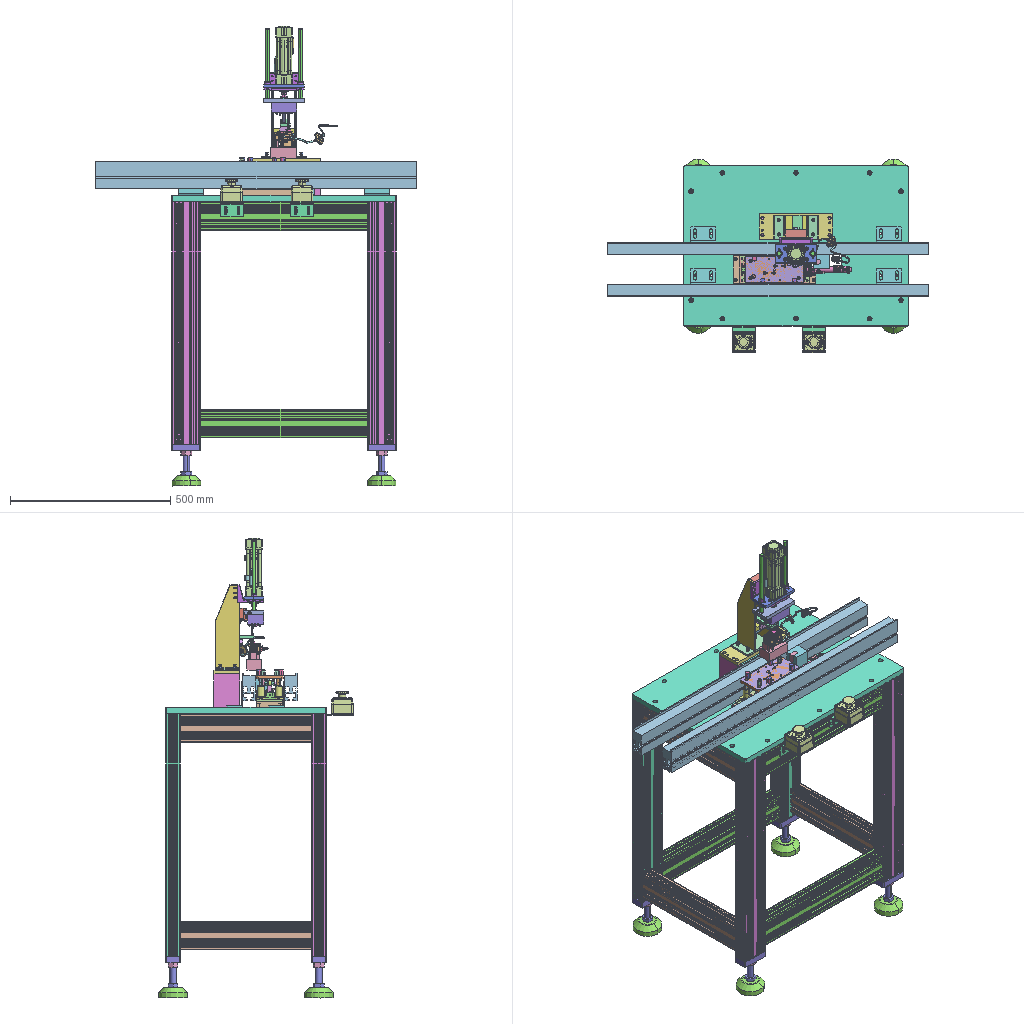Assembly | STEP file | 93 different items | 164 placed | box 1000 x 608 x 1437 mm
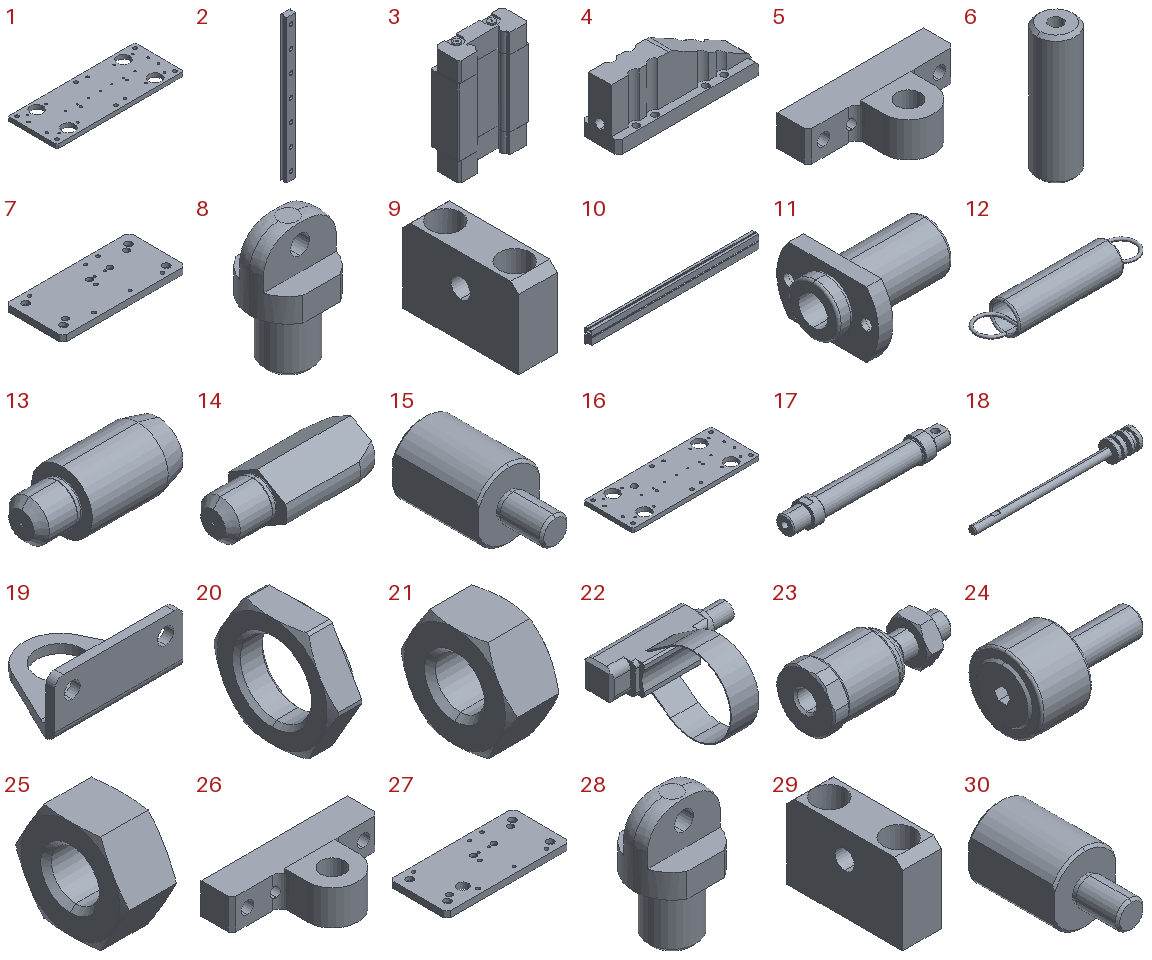Parts list (item | name | quantity | parent item | size | volume):
1 | PN_0007 | x1 | in lifting0012 | 220 x 85 x 7 mm | 118278 mm3
2 | STZL10_135 | x2 | in SE2BZ10_135_SE2BZ10-135 | 9 x 5.5 x 135 mm | 5384 mm3
3 | SEZB10 | x4 | in SE2BZ10_135_SE2BZ10-135 | 20 x 7.8 x 30 mm | 3504 mm3
4 | PN_0032 | x2 | in support001 | 75 x 20 x 31 mm | 24213 mm3
5 | PN_0022 | x1 | in lifting0012 | 38 x 21.5 x 9 mm | 3334 mm3
6 | PSFGT12-40-M5 | x4 | in lifting0012 | 12 x 12 x 40 mm | 4311 mm3
7 | PN_0010 | x1 | in lifting0012 | 180 x 84 x 9 mm | 130838 mm3
8 | PN_0039 | x2 | in lifting0012 | 8 x 7 x 13 mm | 305.811 mm3
9 | PN_0029 | x1 | in lifting0012 | 10 x 30 x 20 mm | 4165 mm3
10 | 8000-001 | x2 | in convvvvv | 1000 x 38.9 x 86 mm | 2174515 mm3
11 | LHICD12_LHICD12 | x8 | in lifting0012, PN_0033 | 47 x 42 x 27 mm | 14694 mm3
12 | AWA6_30_AWA6-30 | x3 | in lifting0012, PN_0033 | 31.1 x 6 x 6 mm | 196.407 mm3
13 | FPBA8_P12_L9_B15_FPBA8-P12-L8-B15 | x2 | in lifting0012, PN_0033 | 27 x 12 x 12 mm | 2448 mm3
14 | FPBD8_P12_L9_B15_FPBD8-P12-L9-B15 | x2 | in lifting0012, PN_0033 | 28 x 12 x 10.127 mm | 1917 mm3
15 | PN_0003 | x4 | in lifting0012 | 13 x 28.5 x 15 mm | 3349 mm3
16 | PN_0036 | x1 | in PN_0033 | 220 x 85 x 7 mm | 117728 mm3
17 | 16MALB50_Body | x1 | - | 142 x 21 x 21 mm | 18560 mm3
18 | 16LBMA50_Rod | x1 | - | 128 x 15.5 x 15.5 mm | 5968 mm3
19 | - | x1 | - | 44 x 32.5 x 19 mm | 4333 mm3
20 | 16_MA_Nut | x2 | - | 6 x 25 x 22 mm | 1467 mm3
21 | 16_MA_Nut1 | x1 | - | 5 x 11.547 x 10 mm | 331.027 mm3
22 | CS1_M_S16 | x2 | - | 30 x 26.6 x 17.8 mm | 1348 mm3
23 | F_M06100F_F-M06100F-P | x1 | in pull cylinder16 | 34.5 x 14.8 x 14 mm | 3405 mm3
24 | CFA6_16body | x1 | in CFA6_16_CFA6-16 | 28 x 16 x 16 mm | 2741 mm3
25 | nut_cua_6 | x1 | in CFA6_16_CFA6-16 | 5.2 x 11.547 x 10 mm | 345.699 mm3
26 | PN_0009 | x1 | in PN_0033 | 38 x 21.5 x 9 mm | 3334 mm3
27 | PN_0034 | x1 | in PN_0033 | 180 x 84 x 9 mm | 129247 mm3
28 | PN_0025 | x4 | in PN_0033 | 8 x 7 x 13 mm | 302.267 mm3
29 | PN_0030 | x1 | in PN_0033 | 10 x 30 x 20 mm | 4165 mm3
30 | PN_0015 | x4 | in PN_0033 | 13 x 28.5 x 15 mm | 3349 mm3
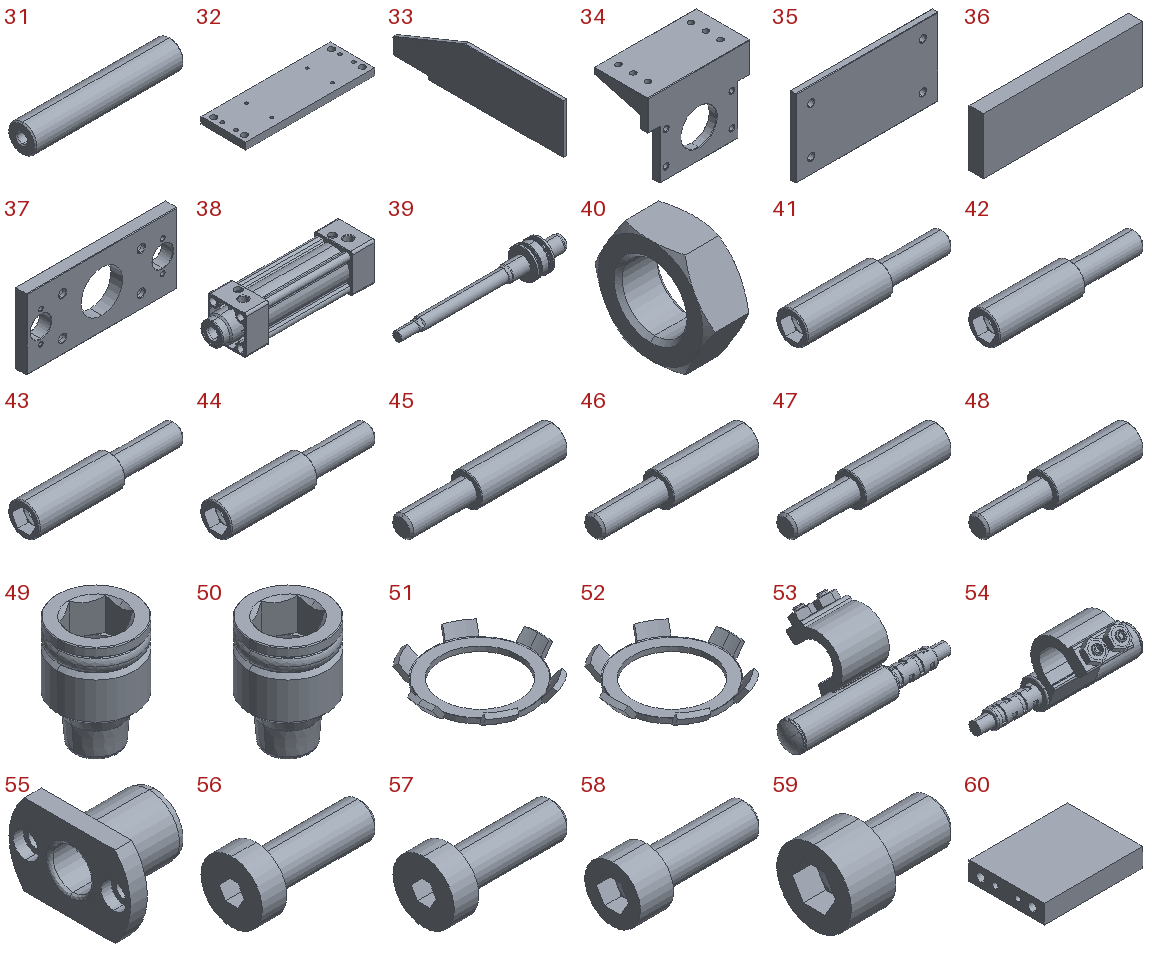31 | PSFGT12_64_M5_PSFGT12-64-M5 | x4 | in PN_0033 | 64 x 12 x 12 mm | 7075 mm3
32 | PN_0023 | x1 | in 10_ASM | 230 x 80 x 12 mm | 214344 mm3
33 | 1002 | x2 | in 10_ASM | - | -
34 | 1003 | x1 | in 10_ASM | 104 x 55 x 81 mm | 80858 mm3
35 | 10040 | x1 | in 10_ASM | 138 x 6 x 75 mm | 61187 mm3
36 | 1005 | x1 | in 10_ASM | 68 x 6 x 24 mm | 9792 mm3
37 | 1006 | x1 | in 10_ASM | 128 x 10 x 60 mm | 58293 mm3
38 | SI-40X75-S-B1N-2-1 | x1 | in SI-40X75-S-B1N-2_ASM | 204.5 x 53 x 53 mm | 210149 mm3
39 | SI-40X75-S-B1N-2-2 | x1 | in SI-40X75-S-B1N-2_ASM | 220.5 x 39.5 x 39.5 mm | 58608 mm3
40 | SI-40X75-S-B1N-2-3 | x1 | in SI-40X75-S-B1N-2_ASM | 7 x 19.63 x 17 mm | 1102 mm3
41 | SI-40X75-S-B1N-2-4 | x1 | in SI-40X75-S-B1N-2_ASM | 43 x 9 x 9 mm | 1649 mm3
42 | SI-40X75-S-B1N-2-5 | x1 | in SI-40X75-S-B1N-2_ASM | 43 x 9 x 9 mm | 1649 mm3
43 | SI-40X75-S-B1N-2-6 | x1 | in SI-40X75-S-B1N-2_ASM | 43 x 9 x 9 mm | 1649 mm3
44 | SI-40X75-S-B1N-2-7 | x1 | in SI-40X75-S-B1N-2_ASM | 43 x 9 x 9 mm | 1649 mm3
45 | SI-40X75-S-B1N-2-8 | x1 | in SI-40X75-S-B1N-2_ASM | 43 x 9 x 9 mm | 1649 mm3
46 | SI-40X75-S-B1N-2-9 | x1 | in SI-40X75-S-B1N-2_ASM | 43 x 9 x 9 mm | 1649 mm3
47 | SI-40X75-S-B1N-2-10 | x1 | in SI-40X75-S-B1N-2_ASM | 43 x 9 x 9 mm | 1649 mm3
48 | SI-40X75-S-B1N-2-11 | x1 | in SI-40X75-S-B1N-2_ASM | 43 x 9 x 9 mm | 1649 mm3
49 | SI-40X75-S-B1N-2-12 | x1 | in SI-40X75-S-B1N-2_ASM | 10 x 10 x 14.13 mm | 659.781 mm3
50 | SI-40X75-S-B1N-2-13 | x1 | in SI-40X75-S-B1N-2_ASM | 10 x 10 x 14.13 mm | 659.781 mm3
51 | SI-40X75-S-B1N-2-14 | x1 | in SI-40X75-S-B1N-2_ASM | 10 x 9.485 x 1.224 mm | 14.035 mm3
52 | SI-40X75-S-B1N-2-15 | x1 | in SI-40X75-S-B1N-2_ASM | 10 x 9.485 x 1.224 mm | 14.035 mm3
53 | SI-40X75-S-B1N-2-16 | x1 | in SI-40X75-S-B1N-2_ASM | 53.8 x 23.917 x 26.321 mm | 4702 mm3
54 | SI-40X75-S-B1N-2-17 | x1 | in SI-40X75-S-B1N-2_ASM | 53.8 x 23.917 x 26.321 mm | 4702 mm3
55 | SHTNZ12-25_1 | x2 | - | 25 x 36 x 24 mm | 5866 mm3
56 | SHTNZ12-25_2 | x2 | - | 14.8 x 7 x 7 mm | 244.398 mm3
57 | SHTNZ12-25_3 | x2 | - | 14.8 x 7 x 7 mm | 244.398 mm3
58 | CB6X1-L18-A10-E6-B5 | x6 | in 10_ASM, 20_ASM | 24 x 10 x 10 mm | 907.535 mm3
59 | CB6X1-10-A10-E6-B5 | x4 | in 10_ASM | 16 x 10 x 10 mm | 681.341 mm3
60 | PN_0028 | x2 | in 10_ASM | 105 x 80 x 20 mm | 160821 mm3
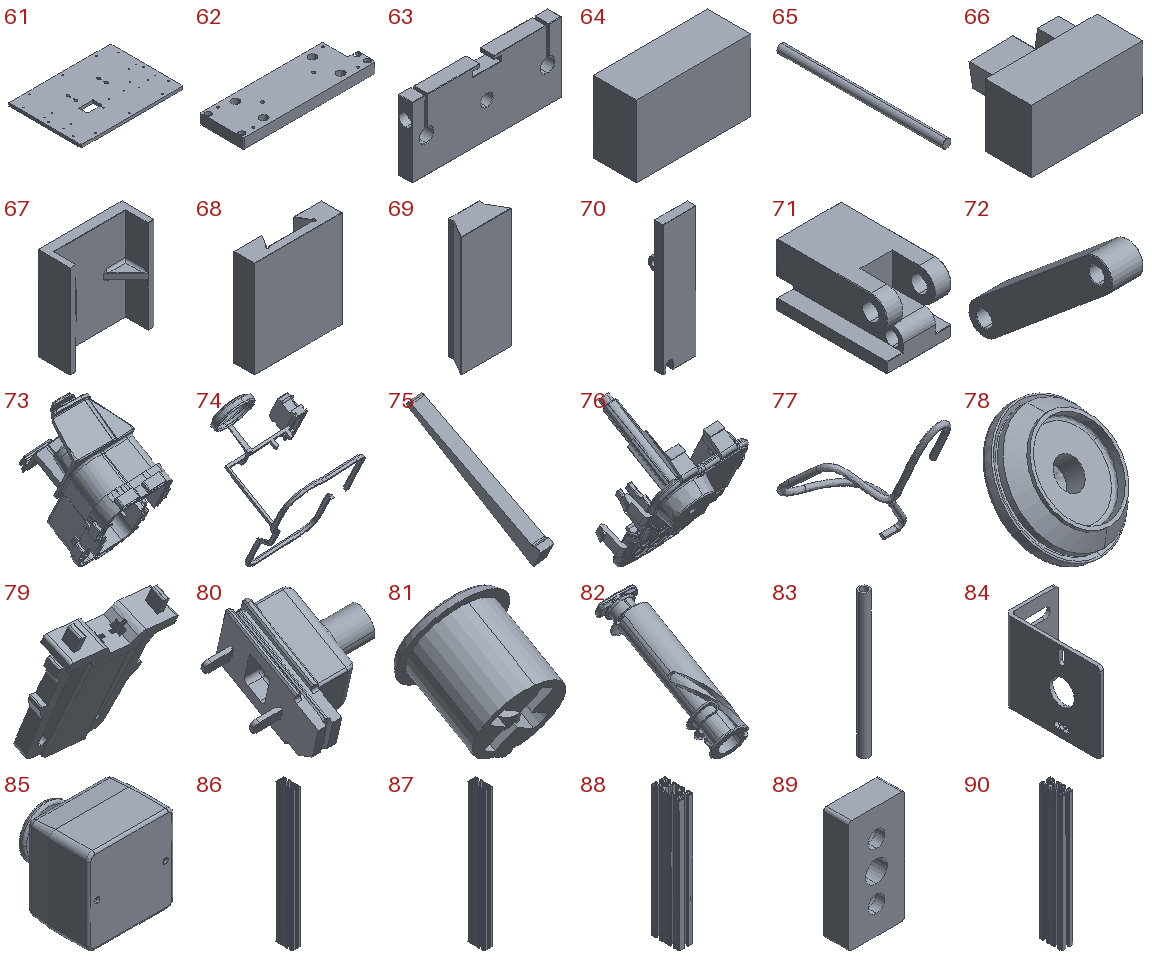61 | PN_0004 | x1 | in 10_ASM | 700 x 500 x 20 mm | 6828580 mm3
62 | PN_0024 | x1 | in 10_ASM | 258 x 85 x 19.5 mm | 387959 mm3
63 | 2001 | x1 | in 20_ASM | - | -
64 | 2000-01 | x1 | in 20_ASM | 80 x 30 x 50 mm | 120000 mm3
65 | 2002 | x2 | in 20_ASM | 12 x 230 x 12 mm | 26009 mm3
66 | 2004 | x1 | in 20_ASM | 80 x 56 x 45 mm | 134107 mm3
67 | 2005 | x1 | in 20_ASM | 68 x 26 x 75 mm | 56012 mm3
68 | 2006 | x1 | in 20_ASM | 68 x 16 x 75 mm | 58521 mm3
69 | 2007 | x1 | in 20_ASM | 35.8 x 15.999 x 85 mm | 37123 mm3
70 | 2008 | x1 | in 20_ASM | 30.6 x 22.5 x 120 mm | 30242 mm3
71 | 2009 | x1 | in 20_ASM | 24 x 41 x 23 mm | 16072 mm3
72 | 2010 | x1 | in 20_ASM | 12 x 54.895 x 48 mm | 8735 mm3
73 | PN_0008 | x1 | in PN_0019 | - | -
74 | PN_0017 | x1 | in PN_0019 | - | -
75 | PN_0037 | x1 | in PN_0019 | 2.149 x 18.473 x 10.911 mm | 52.704 mm3
76 | PN_0002 | x2 | in PN_0011, press_assembly_machineasm | 44.212 x 45.623 x 60.394 mm | 5607 mm3
77 | PN_0031 | x1 | in PN_0035 | 108.679 x 96.834 x 151.567 mm | 5490 mm3
78 | PN_0005 | x1 | in PN_0035 | 37.79 x 29.078 x 30.931 mm | 7006 mm3
79 | PN_0018 | x1 | in PN_0035 | - | -
80 | PN_0016 | x1 | in PN_0035 | 24.961 x 26.123 x 19.511 mm | 2436 mm3
81 | PN_0040 | x2 | in PN_0042 | - | -
82 | PN_0041 | x2 | in PN_0042 | - | -
83 | Spring | x1 | in press_assembly_machineasm | 6.3 x 6.3 x 88.5 mm | 1474 mm3
84 | PN_0021 | x2 | in PN_0012 | - | -
85 | stop_-005 | x2 | in PN_0012 | 68 x 70 x 68 mm | 54810 mm3
86 | PN_0014 | x2 | in PN_0001 | 45 x 90 x 757.5 mm | 975869 mm3
87 | PN_0020 | x2 | in PN_0001 | 45 x 90 x 757.5 mm | 985388 mm3
88 | PN_0026 | x4 | in PN_0001 | 45 x 90 x 410 mm | 533346 mm3
89 | PN_0027 | x4 | in PN_0001 | 45 x 20 x 90 mm | 65910 mm3
90 | PN_0006 | x4 | in PN_0001 | 45 x 90 x 520 mm | 676438 mm3
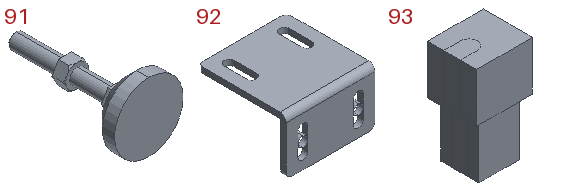91 | FBR90_20_130-005 | x4 | in PN_0001 | - | -
92 | PN_0038 | x4 | - | - | -
93 | 00000 | x1 | - | 50 x 44 x 94 mm | 158000 mm3
Placements (level | parent | child | x y z in mm | rotation matrix by rows):
1 | subassembly 2 | lifting0012 | 28.438 4.92 -155.671 | 1 -2e-06 0 -2e-06 -1 0 0 0 -1
2 | lifting0012 | PN_0007 | -10.26 -1.954 -4.0 | 1 0 0 0 1 0 0 0 1
2 | lifting0012 | support001 | -2.76 -6.648 -10.036 | 0 0 1 -1 0 0 0 -1 -0
3 | support001 | SE2BZ10_135_SE2BZ10-135 | -4.693 -6.036 -67.5 | 1 0 0 0 1 0 0 0 1
4 | SE2BZ10_135_SE2BZ10-135 | STZL10_135 | 0.0 0.0 -0.0 | 1 0 0 0 1 0 0 0 1
4 | SE2BZ10_135_SE2BZ10-135 | SEZB10 | 0.0 2.2 57.0 | 1 0 0 0 1 0 0 0 1
4 | SE2BZ10_135_SE2BZ10-135 | SEZB10 | 0.0 2.2 20.0 | 1 0 0 0 1 0 0 0 1
3 | support001 | PN_0032 | -4.693 3.964 -27.0 | 0 1 0 0 0 1 1 0 0
2 | lifting0012 | PN_0022 | 6.24 -16.954 -53.0 | 1 0 0 0 0 1 0 -1 -0
2 | lifting0012 | PSFGT12-40-M5 | -85.26 25.546 -28.0 | -0.7613 0.6484 0 0.6484 0.7613 0 0 0 -1
2 | lifting0012 | PSFGT12-40-M5 | 64.74 -29.454 -28.0 | -0.7317 -0.6816 0 -0.6816 0.7317 0 0 0 -1
2 | lifting0012 | PSFGT12-40-M5 | -85.26 -29.454 -28.0 | -0.7636 -0.6457 0 -0.6457 0.7636 0 0 0 -1
2 | lifting0012 | PSFGT12-40-M5 | 64.74 25.546 -28.0 | -0.7613 0.6484 0 0.6484 0.7613 0 0 0 -1
2 | lifting0012 | PN_0010 | -10.26 -1.954 -68.0 | 1 0 0 0 -1 0 0 0 -1
2 | lifting0012 | PN_0039 | 7.24 30.546 -74.0 | -0.8847 0.4662 0 -0.4662 -0.8847 0 0 0 1
2 | lifting0012 | PN_0039 | 7.24 30.546 2.0 | 0.9539 -0.3003 0 -0.3003 -0.9539 0 0 0 -1
2 | lifting0012 | PN_0029 | 2667.74 0.5456 -4.0 | -1 0 0 0 1 0 0 0 -1
2 | lifting0012 | convvvvv | 245.368 56.193 -42.0 | 1 0 0 0 1 0 0 0 1
3 | convvvvv | 8000-001 | -276.128 7.403 -3.776 | 1 0 0 0 1 0 0 0 1
3 | convvvvv | 8000-001 | -276.128 -123.697 -3.776 | -1 0 0 0 -1 0 0 0 1
2 | lifting0012 | LHICD12_LHICD12 | 64.74 -29.454 -10.0 | 0 1 0 0 0 -1 -1 0 0
2 | lifting0012 | AWA6_30_AWA6-30 | 7.24 30.546 -41.55 | 0 0 -1 0 1 0 1 0 0
2 | lifting0012 | LHICD12_LHICD12 | 64.74 25.546 -10.0 | 0 1 0 0 0 -1 -1 0 0
2 | lifting0012 | LHICD12_LHICD12 | -85.26 25.546 -10.0 | 0 1 0 0 0 -1 -1 0 0
2 | lifting0012 | LHICD12_LHICD12 | -85.26 -29.454 -10.0 | 0 1 0 0 0 -1 -1 0 0
2 | lifting0012 | FPBA8_P12_L9_B15_FPBA8-P12-L8-B15 | -75.76 19.046 -77.0 | 0 0 1 0 1 0 -1 0 0
2 | lifting0012 | FPBD8_P12_L9_B15_FPBD8-P12-L9-B15 | 55.24 -22.954 -77.0 | 0 0 1 0 1 0 -1 0 0
2 | lifting0012 | PN_0003 | 52.74 32.046 -77.0 | 1 0 0 0 0 1 0 -1 -0
2 | lifting0012 | PN_0003 | -47.26 32.046 -77.0 | 1 0 0 0 0 1 0 -1 -0
2 | lifting0012 | PN_0003 | -73.26 -35.954 -77.0 | -0.971 0 -0.2389 0.2389 0 -0.971 0 -1 0
2 | lifting0012 | PN_0003 | 26.74 -35.954 -77.0 | 1 0 0 0 0 1 0 -1 -0
2 | lifting0012 | PN_0033 | -20.521 -3.909 -0.0 | -1 0 0 0 -1 0 0 0 1
3 | PN_0033 | PN_0036 | -10.26 -1.954 -4.0 | 1 0 0 0 1 0 0 0 1
3 | PN_0033 | support001 | -2.76 -6.648 -10.036 | 0 0 1 -1 0 0 0 -1 0
4 | support001 | SE2BZ10_135_SE2BZ10-135 | -4.693 -6.036 -67.5 | 1 0 0 0 1 0 0 0 1
5 | SE2BZ10_135_SE2BZ10-135 | STZL10_135 | 0.0 0.0 -0.0 | 1 0 0 0 1 0 0 0 1
5 | SE2BZ10_135_SE2BZ10-135 | SEZB10 | 0.0 2.2 57.0 | 1 0 0 0 1 0 0 0 1
5 | SE2BZ10_135_SE2BZ10-135 | SEZB10 | 0.0 2.2 20.0 | 1 0 0 0 1 0 0 0 1
4 | support001 | PN_0032 | -4.693 3.964 -27.0 | 0 1 0 0 0 1 1 0 0
3 | PN_0033 | pull cylinder16 | -177.286 -1.954 -33.923 | -1 0 0 0 0 -1 0 -1 -0
4 | pull cylinder16 | subassembly 3 | -43.025 -9.923 -0.0 | 1 0 0 0 1 0 0 0 1
5 | subassembly 3 | 16MALB50_Body | -26.0 0.0 0.0 | 1 0 0 0 1 0 0 0 1
5 | subassembly 3 | 16LBMA50_Rod | -48.0 0.0 0.0 | 1 0 0 0 1 0 0 0 1
5 | subassembly 3 | subassembly 4 | -10.0 -0.0 0.0 | 0 0 -1 0 1 0 1 0 0
5 | subassembly 3 | 16_MA_Nut | -19.0 0.0 0.0 | 1 0 0 0 1 0 0 0 1
5 | subassembly 3 | 16_MA_Nut1 | -40.0 0.0 0.0 | -1 0 0 0 -1 0 0 0 1
5 | subassembly 3 | CS1_M_S16 | 1.0 0.0 0.0 | 1 0 0 0 0.7071 -0.7071 0 0.7071 0.7071
5 | subassembly 3 | CS1_M_S16 | 89.0 0.0 0.0 | -1 0 0 0 0.7071 -0.7071 0 -0.7071 -0.7071
5 | subassembly 3 | 16_MA_Nut | 109.0 0.0 0.0 | -1 0 0 0 -1 0 0 0 1
4 | pull cylinder16 | F_M06100F_F-M06100F-P | -81.025 -9.923 -0.0 | -1 0 0 0 0.9783 0.2073 0 0.2073 -0.9783
3 | PN_0033 | CFA6_16_CFA6-16 | 6.24 -7.954 -53.0 | 0 0.7346 0.6785 -1 0 0 0 -0.6785 0.7346
4 | CFA6_16_CFA6-16 | CFA6_16body | -0.0 -0.0 -0.0 | 1 0 0 0 1 0 0 0 1
4 | CFA6_16_CFA6-16 | nut_cua_6 | 11.5 0.0 -0.0 | -1 0 0 0 -1 0 0 0 1
3 | PN_0033 | PN_0009 | 6.24 -16.954 -53.0 | 1 0 0 0 0 1 0 -1 -0
3 | PN_0033 | PN_0034 | -10.26 -1.954 -68.0 | 1 0 0 0 -1 0 0 0 -1
3 | PN_0033 | PN_0025 | 7.24 30.546 -74.0 | -0.8847 0.4662 0 -0.4662 -0.8847 0 0 0 1
3 | PN_0033 | PN_0025 | 7.24 30.546 2.0 | 0.9539 -0.3003 0 -0.3003 -0.9539 0 0 0 -1
3 | PN_0033 | PN_0025 | 7.24 -34.454 2.0 | 0.9539 -0.3003 0 -0.3003 -0.9539 0 0 0 -1
3 | PN_0033 | PN_0025 | 7.24 -34.454 -74.0 | -0.8847 0.4662 0 -0.4662 -0.8847 0 0 0 1
3 | PN_0033 | PN_0030 | 2667.74 0.5456 -4.0 | -1 0 0 0 1 0 0 0 -1
3 | PN_0033 | LHICD12_LHICD12 | 64.74 -29.454 -10.0 | 0 1 0 0 0 -1 -1 0 -0
3 | PN_0033 | AWA6_30_AWA6-30 | 7.24 30.546 -41.55 | 0 0.01636 -0.9999 0 0.9999 0.01636 1 0 0
3 | PN_0033 | AWA6_30_AWA6-30 | 7.24 -34.454 -41.55 | 0 0.01636 -0.9999 0 0.9999 0.01636 1 0 0
3 | PN_0033 | LHICD12_LHICD12 | 64.74 25.546 -10.0 | 0 1 0 0 0 -1 -1 0 -0
3 | PN_0033 | LHICD12_LHICD12 | -85.26 25.546 -10.0 | 0 1 0 0 0 -1 -1 0 -0
3 | PN_0033 | LHICD12_LHICD12 | -85.26 -29.454 -10.0 | 0 1 0 0 0 -1 -1 0 -0
3 | PN_0033 | FPBA8_P12_L9_B15_FPBA8-P12-L8-B15 | -75.76 19.046 -77.0 | 0 0 1 0 1 0 -1 0 0
3 | PN_0033 | FPBD8_P12_L9_B15_FPBD8-P12-L9-B15 | 55.24 -22.954 -77.0 | 0 0 1 0 1 0 -1 0 0
3 | PN_0033 | PN_0015 | 52.74 32.046 -77.0 | 1 0 0 0 0 1 0 -1 -0
3 | PN_0033 | PN_0015 | -47.26 32.046 -77.0 | 1 0 0 0 0 1 0 -1 -0
3 | PN_0033 | PN_0015 | -73.26 -35.954 -77.0 | -0.971 0 -0.2389 0.2389 0 -0.971 0 -1 0
3 | PN_0033 | PN_0015 | 26.74 -35.954 -77.0 | 1 0 0 0 0 1 0 -1 -0
3 | PN_0033 | PSFGT12_64_M5_PSFGT12-64-M5 | -85.26 25.546 -68.0 | 0 0.08569 -0.9963 0 0.9963 0.08569 1 0 -0
3 | PN_0033 | PSFGT12_64_M5_PSFGT12-64-M5 | 64.74 25.546 -68.0 | 0 0.08569 -0.9963 0 0.9963 0.08569 1 0 -0
3 | PN_0033 | PSFGT12_64_M5_PSFGT12-64-M5 | 64.74 -29.454 -68.0 | 0 0.487 -0.8734 0 0.8734 0.487 1 0 -0
3 | PN_0033 | PSFGT12_64_M5_PSFGT12-64-M5 | -85.26 -29.454 -68.0 | 0 0.487 -0.8734 0 0.8734 0.487 1 0 -0
1 | subassembly 2 | press_assembly_machineasm | 85.178 96.374 -67.171 | -1 0 2e-06 2e-06 0 1 0 1 0
2 | press_assembly_machineasm | 10_ASM | -0.0 -0.0 -0.0 | 1 0 0 0 1 0 0 0 1
3 | 10_ASM | PN_0023 | -0.0 6.0 45.0 | 1 0 0 0 0 -1 0 1 0
3 | 10_ASM | 1002 | -0.0 -0.0 -0.0 | 1 0 0 0 1 0 0 0 1
3 | 10_ASM | 1002 | -74.0 -0.0 -0.0 | 1 0 0 0 1 0 0 0 1
3 | 10_ASM | 1003 | -0.0 -0.0 -0.0 | 1 0 0 0 1 0 0 0 1
3 | 10_ASM | 10040 | -0.0 -6.0 -0.0 | 1 0 0 0 1 0 0 0 1
3 | 10_ASM | 1005 | -0.0 -0.0 -0.0 | 1 0 0 0 1 0 0 0 1
3 | 10_ASM | 1006 | -0.0 -0.0 -0.0 | 1 0 0 0 1 0 0 0 1
3 | 10_ASM | SI-40X75-S-B1N-2_ASM | 0.0 235.0 -40.0 | 0 -1 0 1 0 0 0 0 1
4 | SI-40X75-S-B1N-2_ASM | SI-40X75-S-B1N-2-1 | 0.0 0.0 -0.0 | 1 0 0 0 1 0 0 0 1
4 | SI-40X75-S-B1N-2_ASM | SI-40X75-S-B1N-2-2 | 0.0 0.0 -0.0 | 1 0 0 0 1 0 0 0 1
4 | SI-40X75-S-B1N-2_ASM | SI-40X75-S-B1N-2-3 | 0.0 0.0 -0.0 | 1 0 0 0 1 0 0 0 1
4 | SI-40X75-S-B1N-2_ASM | SI-40X75-S-B1N-2-4 | 0.0 0.0 -0.0 | 1 0 0 0 1 0 0 0 1
4 | SI-40X75-S-B1N-2_ASM | SI-40X75-S-B1N-2-5 | 0.0 0.0 -0.0 | 1 0 0 0 1 0 0 0 1
4 | SI-40X75-S-B1N-2_ASM | SI-40X75-S-B1N-2-6 | 0.0 0.0 -0.0 | 1 0 0 0 1 0 0 0 1
4 | SI-40X75-S-B1N-2_ASM | SI-40X75-S-B1N-2-7 | 0.0 0.0 -0.0 | 1 0 0 0 1 0 0 0 1
4 | SI-40X75-S-B1N-2_ASM | SI-40X75-S-B1N-2-8 | 0.0 0.0 -0.0 | 1 0 0 0 1 0 0 0 1
4 | SI-40X75-S-B1N-2_ASM | SI-40X75-S-B1N-2-9 | 0.0 0.0 -0.0 | 1 0 0 0 1 0 0 0 1
4 | SI-40X75-S-B1N-2_ASM | SI-40X75-S-B1N-2-10 | 0.0 0.0 -0.0 | 1 0 0 0 1 0 0 0 1
4 | SI-40X75-S-B1N-2_ASM | SI-40X75-S-B1N-2-11 | 0.0 0.0 -0.0 | 1 0 0 0 1 0 0 0 1
4 | SI-40X75-S-B1N-2_ASM | SI-40X75-S-B1N-2-12 | 0.0 0.0 -0.0 | 1 0 0 0 1 0 0 0 1
4 | SI-40X75-S-B1N-2_ASM | SI-40X75-S-B1N-2-13 | 0.0 0.0 -0.0 | 1 0 0 0 1 0 0 0 1
4 | SI-40X75-S-B1N-2_ASM | SI-40X75-S-B1N-2-14 | 0.0 0.0 -0.0 | 1 0 0 0 1 0 0 0 1
4 | SI-40X75-S-B1N-2_ASM | SI-40X75-S-B1N-2-15 | 0.0 0.0 -0.0 | 1 0 0 0 1 0 0 0 1
4 | SI-40X75-S-B1N-2_ASM | SI-40X75-S-B1N-2-16 | 0.0 0.0 -0.0 | 1 0 0 0 1 0 0 0 1
4 | SI-40X75-S-B1N-2_ASM | SI-40X75-S-B1N-2-17 | 0.0 0.0 -0.0 | 1 0 0 0 1 0 0 0 1
3 | 10_ASM | subassembly 5 | -52.0 220.0 -40.0 | 0 0 1 1 0 0 0 1 -0
4 | subassembly 5 | SHTNZ12-25_1 | 0.0 -0.0 -0.0 | 1 0 0 0 1 0 0 0 1
4 | subassembly 5 | SHTNZ12-25_2 | 0.0 -0.0 -0.0 | 1 0 0 0 1 0 0 0 1
4 | subassembly 5 | SHTNZ12-25_3 | 0.0 -0.0 -0.0 | 1 0 0 0 1 0 0 0 1
3 | 10_ASM | subassembly 5 | 52.0 220.0 -40.0 | 0 0 -1 1 0 0 0 -1 0
4 | subassembly 5 | SHTNZ12-25_1 | 0.0 -0.0 -0.0 | 1 0 0 0 1 0 0 0 1
4 | subassembly 5 | SHTNZ12-25_2 | 0.0 -0.0 -0.0 | 1 0 0 0 1 0 0 0 1
4 | subassembly 5 | SHTNZ12-25_3 | 0.0 -0.0 -0.0 | 1 0 0 0 1 0 0 0 1
3 | 10_ASM | CB6X1-L18-A10-E6-B5 | 54.0 18.0 20.0 | 0 1 0 -1 0 0 0 0 1
3 | 10_ASM | CB6X1-L18-A10-E6-B5 | 54.0 18.0 65.0 | 0 1 0 -1 0 0 0 0 1
3 | 10_ASM | CB6X1-L18-A10-E6-B5 | -54.0 18.0 65.0 | 0 1 0 -1 0 0 0 0 1
3 | 10_ASM | CB6X1-L18-A10-E6-B5 | -54.0 18.0 20.0 | 0 1 0 -1 0 0 0 0 1
3 | 10_ASM | CB6X1-10-A10-E6-B5 | 33.5 228.0 -58.0 | 0 1 0 -1 0 0 0 0 1
3 | 10_ASM | CB6X1-10-A10-E6-B5 | 33.5 228.0 -25.0 | 0 1 0 -1 0 0 0 0 1
3 | 10_ASM | CB6X1-10-A10-E6-B5 | -33.5 228.0 -58.0 | 0 1 0 -1 0 0 0 0 1
3 | 10_ASM | CB6X1-10-A10-E6-B5 | -33.5 228.0 -25.0 | 0 1 0 -1 0 0 0 0 1
3 | 10_ASM | PN_0028 | 115.0 -111.0 85.0 | 0 0 -1 1 0 0 0 -1 0
3 | 10_ASM | PN_0028 | -95.0 -111.0 85.0 | 0 0 -1 1 0 0 0 -1 0
3 | 10_ASM | PN_0004 | -350.0 -111.0 -265.0 | 1 0 0 0 0 -1 0 1 0
3 | 10_ASM | PN_0024 | 196.0 -111.0 -132.0 | -1 0 0 0 0 1 0 1 -0
2 | press_assembly_machineasm | 20_ASM | 0.0 -1.598 -0.0 | 1 0 0 0 1 0 0 0 1
3 | 20_ASM | 2001 | 0.0 0.0 0.0 | 1 0 0 0 1 0 0 0 1
3 | 20_ASM | 2000-01 | 0.0 0.0 0.0 | 1 0 0 0 1 0 0 0 1
3 | 20_ASM | 2002 | 0.0 0.0 0.0 | 1 0 0 0 1 0 0 0 1
3 | 20_ASM | 2002 | 104.0 0.0 0.0 | 1 0 0 0 1 0 0 0 1
3 | 20_ASM | CB6X1-L18-A10-E6-B5 | -57.5 187.0 -26.0 | 1 0 0 0 1 0 0 0 1
3 | 20_ASM | CB6X1-L18-A10-E6-B5 | 57.5 187.0 -26.0 | -1 0 0 0 -1 0 0 0 1
3 | 20_ASM | 2004 | 0.0 0.0 0.0 | 1 0 0 0 1 0 0 0 1
3 | 20_ASM | 2005 | 0.0 0.0 0.0 | 1 0 0 0 1 0 0 0 1
3 | 20_ASM | 2006 | 0.0 0.0 0.0 | 1 0 0 0 1 0 0 0 1
3 | 20_ASM | 2007 | 0.0 0.0 0.0 | 1 0 0 0 1 0 0 0 1
3 | 20_ASM | 2008 | 0.0 0.0 0.0 | 1 0 0 0 1 0 0 0 1
3 | 20_ASM | 2009 | 0.0 0.0 0.0 | 1 0 0 0 1 0 0 0 1
3 | 20_ASM | 2010 | 0.0 0.0 0.0 | 1 0 0 0 1 0 0 0 1
2 | press_assembly_machineasm | PN_0013 | -392.029 980.008 2650.126 | 0.175 0.4968 -0.85 -0.004208 -0.863 -0.5053 -0.9846 0.09201 -0.149
3 | PN_0013 | PN_0011 | 13.124 -34.773 -38.37 | 1 0 0 0 1 0 0 0 1
4 | PN_0011 | PN_0019 | -0.0 -0.0 0.0 | 1 0 0 0 1 0 0 0 1
5 | PN_0019 | PN_0008 | 0.0 0.0 -0.0 | 1 0 0 0 1 0 0 0 1
5 | PN_0019 | PN_0017 | 0.0 0.0 -0.0 | 1 0 0 0 1 0 0 0 1
5 | PN_0019 | PN_0037 | 0.0 0.0 -0.0 | 1 0 0 0 1 0 0 0 1
4 | PN_0011 | PN_0002 | -0.0 -0.0 0.0 | 1 0 0 0 1 0 0 0 1
4 | PN_0011 | PN_0035 | 39.059 -123.127 -194.218 | 0.9958 -0.09128 -0.001939 0.09025 0.9874 -0.13 0.01378 0.1293 0.9915
5 | PN_0035 | PN_0031 | 0.0 -0.0 -0.0 | 1 0 0 0 1 0 0 0 1
5 | PN_0035 | PN_0005 | 0.0 -0.0 -0.0 | 1 0 0 0 1 0 0 0 1
5 | PN_0035 | PN_0018 | 0.0 -0.0 -0.0 | 1 0 0 0 1 0 0 0 1
5 | PN_0035 | PN_0016 | 0.0 -0.0 -0.0 | 1 0 0 0 1 0 0 0 1
4 | PN_0011 | PN_0042 | 2905.127 1098.989 -2305.504 | 0.03719 0.3908 -0.9197 -0.4262 0.8386 0.3392 0.9039 0.3794 0.1978
5 | PN_0042 | PN_0040 | -0.0 0.0 -0.0 | 1 0 0 0 1 0 0 0 1
5 | PN_0042 | PN_0041 | -0.0 0.0 -0.0 | 1 0 0 0 1 0 0 0 1
4 | PN_0011 | PN_0042 | 37.464 -112.569 -178.652 | 0.9957 -0.09249 0.000941 0.09183 0.9872 -0.1301 0.0111 0.1296 0.9915
5 | PN_0042 | PN_0040 | -0.0 0.0 -0.0 | 1 0 0 0 1 0 0 0 1
5 | PN_0042 | PN_0041 | -0.0 0.0 -0.0 | 1 0 0 0 1 0 0 0 1
2 | press_assembly_machineasm | PN_0002 | -374.392 1094.39 2639.731 | 0.175 0.4968 -0.85 -0.004208 -0.863 -0.5053 -0.9846 0.09201 -0.149
2 | press_assembly_machineasm | Spring | -13.587 75.185 -34.37 | 0.5936 0.8047 0 0 0 1 0.8047 -0.5936 -0
1 | subassembly 2 | PN_0012 | -4782.747 303.688 -321.615 | 1 0 -2e-06 -2e-06 0 -1 0 1 -0
2 | PN_0012 | PN_0021 | 4924.26 122.444 557.303 | 0 0 1 -1 0 0 0 -1 0
2 | PN_0012 | stop_-005 | 4924.26 147.944 523.303 | 1 0 0 0 1 0 0 0 1
2 | PN_0012 | PN_0001 | 5038.64 -634.056 427.303 | 1 0 0 0 1 0 0 0 1
3 | PN_0001 | PN_0014 | 0.0 757.5 -1425.68 | 0 -1 0 0 0 -1 1 0 -0
3 | PN_0001 | PN_0014 | -341.43 757.5 1470.68 | 0 1 0 0 0 -1 -1 0 -0
3 | PN_0001 | PN_0020 | 0.0 757.5 -1880.68 | 0 -1 0 0 0 -1 1 0 -0
3 | PN_0001 | PN_0020 | 610.0 -0.0 1015.681 | 0 -1 0 0 0 1 -1 0 0
3 | PN_0001 | PN_0026 | -1946.395 -410.715 -410.0 | 1 0 0 0 1 0 0 0 1
3 | PN_0001 | PN_0026 | 1604.966 540.715 -410.0 | -1 0 0 0 -1 0 0 0 1
3 | PN_0001 | PN_0027 | -475.715 -0.0 -432.5 | 0 0 -1 0 -1 0 -1 0 -0
3 | PN_0001 | PN_0027 | -475.715 -0.0 22.5 | 0 0 -1 0 -1 0 -1 0 -0
3 | PN_0001 | PN_0027 | 134.285 0.0 22.5 | 0 0 1 0 -1 0 1 0 0
3 | PN_0001 | PN_0027 | 134.285 0.0 -432.5 | 0 0 1 0 -1 0 1 0 0
3 | PN_0001 | PN_0026 | 949.966 1188.215 -410.0 | -1 0 0 0 -1 0 0 0 1
3 | PN_0001 | PN_0026 | -1291.395 236.785 -410.0 | 1 0 0 0 1 0 0 0 1
3 | PN_0001 | PN_0006 | 89.285 -410.715 -1425.68 | 0 0 -1 0 1 0 1 0 -0
3 | PN_0001 | PN_0006 | -430.715 -410.715 1015.681 | 0 0 1 0 1 0 -1 0 0
3 | PN_0001 | PN_0006 | 89.285 236.785 -1880.68 | 0 0 -1 0 1 0 1 0 -0
3 | PN_0001 | PN_0006 | 89.285 236.785 -1425.68 | 0 0 -1 0 1 0 1 0 -0
3 | PN_0001 | FBR90_20_130-005 | -475.715 -130.0 22.5 | 0.9617 0 0.2741 0 1 0 -0.2741 0 0.9617
3 | PN_0001 | FBR90_20_130-005 | 134.285 -130.0 22.5 | 1 0 0 0 1 0 0 0 1
3 | PN_0001 | FBR90_20_130-005 | 134.285 -130.0 -432.5 | 1 0 0 0 1 0 0 0 1
3 | PN_0001 | FBR90_20_130-005 | -475.715 -130.0 -432.5 | 1 0 0 0 1 0 0 0 1
2 | PN_0012 | PN_0021 | 4705.6 122.444 557.303 | 0 0 1 -1 0 0 0 -1 0
2 | PN_0012 | stop_-005 | 4704.1 147.944 523.303 | 1 0 0 0 1 0 0 0 1
1 | subassembly 2 | PN_0038 | -204.822 91.875 -138.171 | 1 0 -2e-06 -2e-06 0 -1 0 1 -0
1 | subassembly 2 | PN_0038 | 375.178 91.874 -138.171 | 1 0 -2e-06 -2e-06 0 -1 0 1 -0
1 | subassembly 2 | PN_0038 | 375.178 -39.226 -138.171 | 1 0 -2e-06 -2e-06 0 -1 0 1 -0
1 | subassembly 2 | PN_0038 | -204.822 -39.225 -138.171 | 1 0 -2e-06 -2e-06 0 -1 0 1 -0
1 | subassembly 2 | 00000 | 163.678 30.974 -173.671 | 1 2e-06 0 -2e-06 1 0 0 0 1